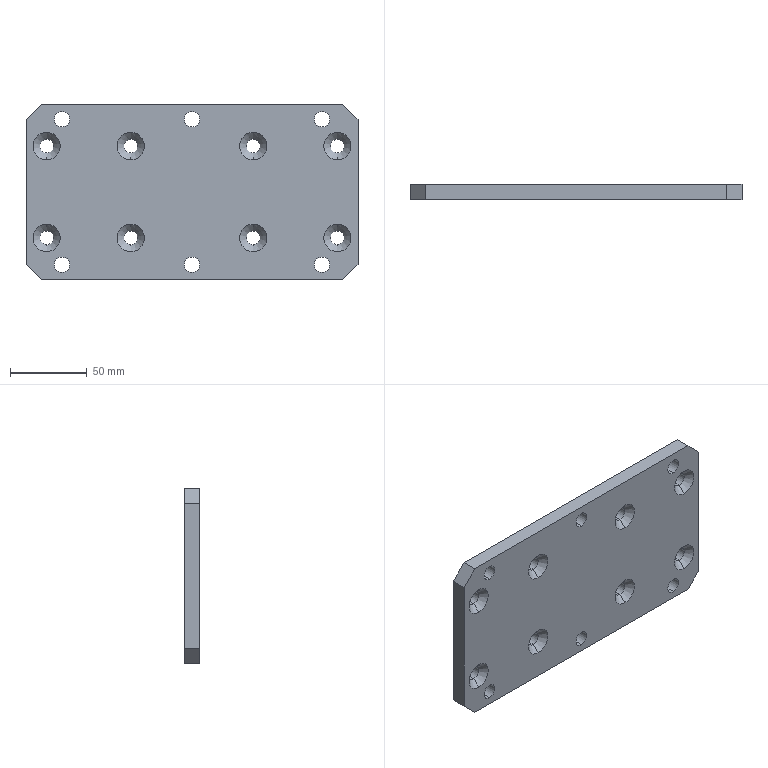Part | SolidWorks | features HoleWzd 2, Chamfer 1, Extrusion 1 | 1 solid | 54 faces | box 217 x 10 x 115 mm | volume 234755 mm3 | cylinder 28 | cone 16 | plane 10 | commonest cylinder face diameters 9 x16 10 x12